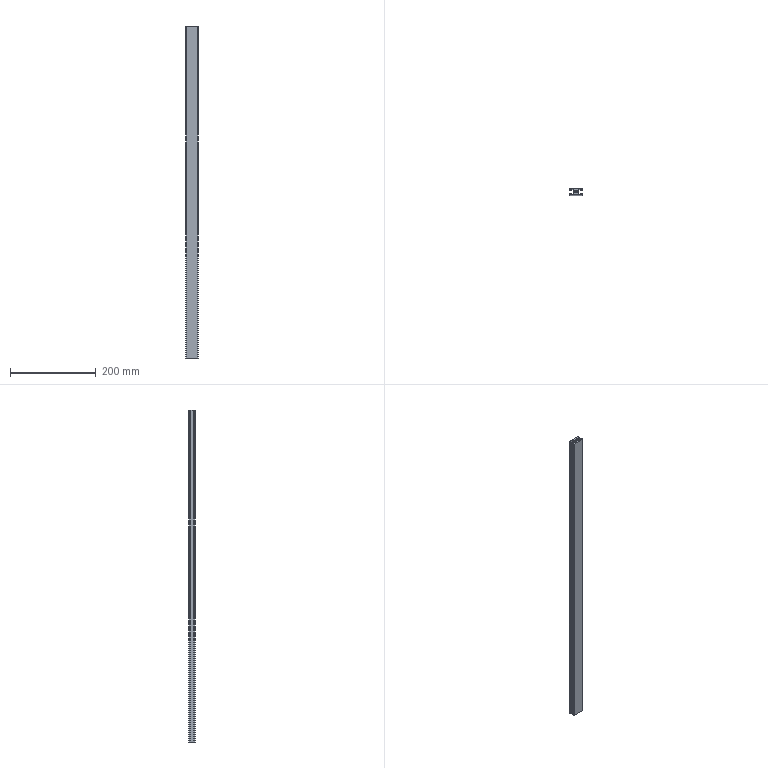Part | SolidWorks | features BaseBody 1, MoveFace 1 | 1 solid | 53 faces | box 30 x 15 x 775 mm | volume 186906 mm3 | plane 38 | cylinder 15 | commonest cylinder face diameters 1 x6 5 x5 2 x4